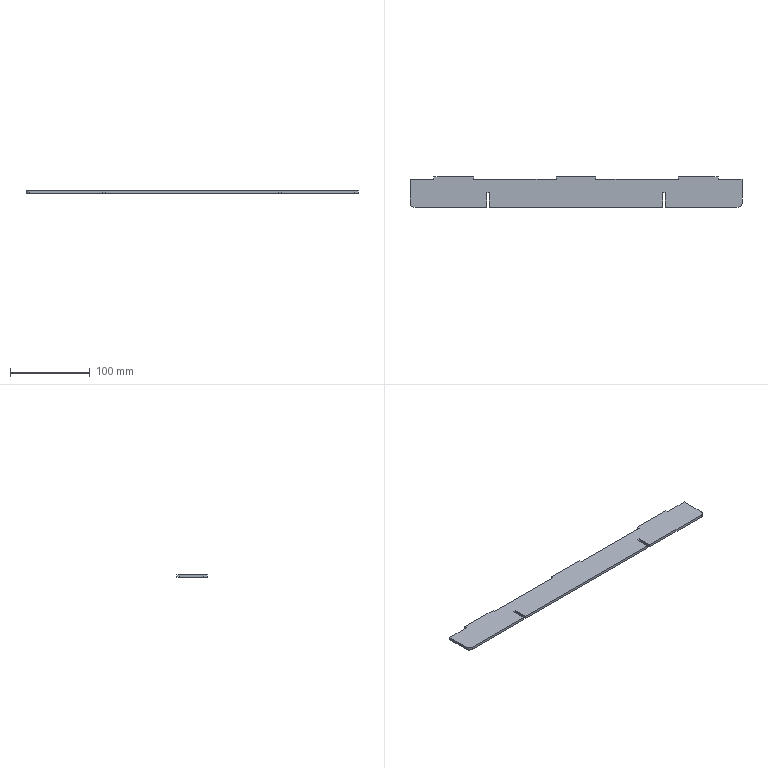Part | SolidWorks | features FlatPattern 1, SMBaseFlange 1, SheetMetal 1 | 1 solid | 28 faces | box 416 x 38 x 3.2 mm | volume 47629 mm3 | plane 26 | cylinder 2 | commonest cylinder face diameters 10 x2
STEP:
#1=CARTESIAN_POINT('',(-198.294,-320.35,0.));
#2=VERTEX_POINT('',#1);
#3=CARTESIAN_POINT('',(-198.294,-350.35,0.));
#4=VERTEX_POINT('',#3);
#5=CARTESIAN_POINT('',(-198.294,-320.35,0.));
#6=DIRECTION('',(0.,-1.,0.));
#7=VECTOR('',#6,1000.);
#8=LINE('',#5,#7);
#9=EDGE_CURVE('',#2,#4,#8,.T.);
#10=ORIENTED_EDGE('',*,*,#9,.F.);
#11=CARTESIAN_POINT('',(-198.294,-320.35,-3.2));
#12=VERTEX_POINT('',#11);
#13=CARTESIAN_POINT('',(-198.294,-320.35,-3.2));
#14=DIRECTION('',(0.,0.,1.));
#15=VECTOR('',#14,1000.);
#16=LINE('',#13,#15);
#17=EDGE_CURVE('',#12,#2,#16,.T.);
#18=ORIENTED_EDGE('',*,*,#17,.F.);
#19=CARTESIAN_POINT('',(-198.294,-350.35,-3.2));
#20=VERTEX_POINT('',#19);
#21=CARTESIAN_POINT('',(-198.294,-320.35,-3.2));
#22=DIRECTION('',(0.,-1.,0.));
#23=VECTOR('',#22,1000.);
#24=LINE('',#21,#23);
#25=EDGE_CURVE('',#12,#20,#24,.T.);
#26=ORIENTED_EDGE('',*,*,#25,.T.);
#27=CARTESIAN_POINT('',(-198.294,-350.35,-3.2));
#28=DIRECTION('',(0.,0.,1.));
#29=VECTOR('',#28,1000.);
#30=LINE('',#27,#29);
#31=EDGE_CURVE('',#20,#4,#30,.T.);
#32=ORIENTED_EDGE('',*,*,#31,.T.);
#33=EDGE_LOOP('',(#10,#18,#26,#32));
#34=FACE_OUTER_BOUND('',#33,.T.);
#35=CARTESIAN_POINT('',(-198.294,-320.35,-3.2));
#36=DIRECTION('',(-1.,0.,0.));
#37=DIRECTION('',(0.,0.,1.));
#38=AXIS2_PLACEMENT_3D('',#35,#36,#37);
#39=PLANE('',#38);
#40=ADVANCED_FACE('',(#34),#39,.T.);
#41=CARTESIAN_POINT('',(-168.294,-320.35,0.));
#42=VERTEX_POINT('',#41);
#43=CARTESIAN_POINT('',(-198.294,-320.35,0.));
#44=DIRECTION('',(-1.,0.,0.));
#45=VECTOR('',#44,1000.);
#46=LINE('',#43,#45);
#47=EDGE_CURVE('',#42,#2,#46,.T.);
#48=ORIENTED_EDGE('',*,*,#47,.F.);
#49=CARTESIAN_POINT('',(-168.294,-320.35,-3.2));
#50=VERTEX_POINT('',#49);
#51=CARTESIAN_POINT('',(-168.294,-320.35,-3.2));
#52=DIRECTION('',(0.,0.,1.));
#53=VECTOR('',#52,1000.);
#54=LINE('',#51,#53);
#55=EDGE_CURVE('',#50,#42,#54,.T.);
#56=ORIENTED_EDGE('',*,*,#55,.F.);
#57=CARTESIAN_POINT('',(-198.294,-320.35,-3.2));
#58=DIRECTION('',(-1.,0.,0.));
#59=VECTOR('',#58,1000.);
#60=LINE('',#57,#59);
#61=EDGE_CURVE('',#50,#12,#60,.T.);
#62=ORIENTED_EDGE('',*,*,#61,.T.);
#63=ORIENTED_EDGE('',*,*,#17,.T.);
#64=EDGE_LOOP('',(#48,#56,#62,#63));
#65=FACE_OUTER_BOUND('',#64,.T.);
#66=CARTESIAN_POINT('',(-198.294,-320.35,-3.2));
#67=DIRECTION('',(0.,1.,0.));
#68=DIRECTION('',(0.,0.,1.));
#69=AXIS2_PLACEMENT_3D('',#66,#67,#68);
#70=PLANE('',#69);
#71=ADVANCED_FACE('',(#65),#70,.T.);
#72=CARTESIAN_POINT('',(-168.294,-317.35,0.));
#73=VERTEX_POINT('',#72);
#74=CARTESIAN_POINT('',(-168.294,-320.35,0.));
#75=DIRECTION('',(0.,-1.,0.));
#76=VECTOR('',#75,1000.);
#77=LINE('',#74,#76);
#78=EDGE_CURVE('',#73,#42,#77,.T.);
#79=ORIENTED_EDGE('',*,*,#78,.F.);
#80=CARTESIAN_POINT('',(-168.294,-317.35,-3.2));
#81=VERTEX_POINT('',#80);
#82=CARTESIAN_POINT('',(-168.294,-317.35,-3.2));
#83=DIRECTION('',(0.,0.,1.));
#84=VECTOR('',#83,1000.);
#85=LINE('',#82,#84);
#86=EDGE_CURVE('',#81,#73,#85,.T.);
#87=ORIENTED_EDGE('',*,*,#86,.F.);
#88=CARTESIAN_POINT('',(-168.294,-320.35,-3.2));
#89=DIRECTION('',(0.,-1.,0.));
#90=VECTOR('',#89,1000.);
#91=LINE('',#88,#90);
#92=EDGE_CURVE('',#81,#50,#91,.T.);
#93=ORIENTED_EDGE('',*,*,#92,.T.);
#94=ORIENTED_EDGE('',*,*,#55,.T.);
#95=EDGE_LOOP('',(#79,#87,#93,#94));
#96=FACE_OUTER_BOUND('',#95,.T.);
#97=CARTESIAN_POINT('',(-168.294,-320.35,-3.2));
#98=DIRECTION('',(-1.,0.,0.));
#99=DIRECTION('',(0.,0.,1.));
#100=AXIS2_PLACEMENT_3D('',#97,#98,#99);
#101=PLANE('',#100);
#102=ADVANCED_FACE('',(#96),#101,.T.);
#103=CARTESIAN_POINT('',(-118.294,-317.35,0.));
#104=VERTEX_POINT('',#103);
#105=CARTESIAN_POINT('',(-168.294,-317.35,0.));
#106=DIRECTION('',(-1.,0.,0.));
#107=VECTOR('',#106,1000.);
#108=LINE('',#105,#107);
#109=EDGE_CURVE('',#104,#73,#108,.T.);
#110=ORIENTED_EDGE('',*,*,#109,.F.);
#111=CARTESIAN_POINT('',(-118.294,-317.35,-3.2));
#112=VERTEX_POINT('',#111);
#113=CARTESIAN_POINT('',(-118.294,-317.35,-3.2));
#114=DIRECTION('',(0.,0.,1.));
#115=VECTOR('',#114,1000.);
#116=LINE('',#113,#115);
#117=EDGE_CURVE('',#112,#104,#116,.T.);
#118=ORIENTED_EDGE('',*,*,#117,.F.);
#119=CARTESIAN_POINT('',(-168.294,-317.35,-3.2));
#120=DIRECTION('',(-1.,0.,0.));
#121=VECTOR('',#120,1000.);
#122=LINE('',#119,#121);
#123=EDGE_CURVE('',#112,#81,#122,.T.);
#124=ORIENTED_EDGE('',*,*,#123,.T.);
#125=ORIENTED_EDGE('',*,*,#86,.T.);
#126=EDGE_LOOP('',(#110,#118,#124,#125));
#127=FACE_OUTER_BOUND('',#126,.T.);
#128=CARTESIAN_POINT('',(-168.294,-317.35,-3.2));
#129=DIRECTION('',(0.,1.,0.));
#130=DIRECTION('',(0.,0.,1.));
#131=AXIS2_PLACEMENT_3D('',#128,#129,#130);
#132=PLANE('',#131);
#133=ADVANCED_FACE('',(#127),#132,.T.);
#134=CARTESIAN_POINT('',(-118.294,-320.35,0.));
#135=VERTEX_POINT('',#134);
#136=CARTESIAN_POINT('',(-118.294,-317.35,0.));
#137=DIRECTION('',(0.,1.,0.));
#138=VECTOR('',#137,1000.);
#139=LINE('',#136,#138);
#140=EDGE_CURVE('',#135,#104,#139,.T.);
#141=ORIENTED_EDGE('',*,*,#140,.F.);
#142=CARTESIAN_POINT('',(-118.294,-320.35,-3.2));
#143=VERTEX_POINT('',#142);
#144=CARTESIAN_POINT('',(-118.294,-320.35,-3.2));
#145=DIRECTION('',(0.,0.,1.));
#146=VECTOR('',#145,1000.);
#147=LINE('',#144,#146);
#148=EDGE_CURVE('',#143,#135,#147,.T.);
#149=ORIENTED_EDGE('',*,*,#148,.F.);
#150=CARTESIAN_POINT('',(-118.294,-317.35,-3.2));
#151=DIRECTION('',(0.,1.,0.));
#152=VECTOR('',#151,1000.);
#153=LINE('',#150,#152);
#154=EDGE_CURVE('',#143,#112,#153,.T.);
#155=ORIENTED_EDGE('',*,*,#154,.T.);
#156=ORIENTED_EDGE('',*,*,#117,.T.);
#157=EDGE_LOOP('',(#141,#149,#155,#156));
#158=FACE_OUTER_BOUND('',#157,.T.);
#159=CARTESIAN_POINT('',(-118.294,-317.35,-3.2));
#160=DIRECTION('',(1.,0.,0.));
#161=DIRECTION('',(0.,1.,0.));
#162=AXIS2_PLACEMENT_3D('',#159,#160,#161);
#163=PLANE('',#162);
#164=ADVANCED_FACE('',(#158),#163,.T.);
#165=CARTESIAN_POINT('',(-15.294,-320.35,0.));
#166=VERTEX_POINT('',#165);
#167=CARTESIAN_POINT('',(-118.294,-320.35,0.));
#168=DIRECTION('',(-1.,0.,0.));
#169=VECTOR('',#168,1000.);
#170=LINE('',#167,#169);
#171=EDGE_CURVE('',#166,#135,#170,.T.);
#172=ORIENTED_EDGE('',*,*,#171,.F.);
#173=CARTESIAN_POINT('',(-15.294,-320.35,-3.2));
#174=VERTEX_POINT('',#173);
#175=CARTESIAN_POINT('',(-15.294,-320.35,-3.2));
#176=DIRECTION('',(0.,0.,1.));
#177=VECTOR('',#176,1000.);
#178=LINE('',#175,#177);
#179=EDGE_CURVE('',#174,#166,#178,.T.);
#180=ORIENTED_EDGE('',*,*,#179,.F.);
#181=CARTESIAN_POINT('',(-118.294,-320.35,-3.2));
#182=DIRECTION('',(-1.,0.,0.));
#183=VECTOR('',#182,1000.);
#184=LINE('',#181,#183);
#185=EDGE_CURVE('',#174,#143,#184,.T.);
#186=ORIENTED_EDGE('',*,*,#185,.T.);
#187=ORIENTED_EDGE('',*,*,#148,.T.);
#188=EDGE_LOOP('',(#172,#180,#186,#187));
#189=FACE_OUTER_BOUND('',#188,.T.);
#190=CARTESIAN_POINT('',(-118.294,-320.35,-3.2));
#191=DIRECTION('',(0.,1.,0.));
#192=DIRECTION('',(0.,0.,1.));
#193=AXIS2_PLACEMENT_3D('',#190,#191,#192);
#194=PLANE('',#193);
#195=ADVANCED_FACE('',(#189),#194,.T.);
#196=CARTESIAN_POINT('',(-15.294,-317.35,0.));
#197=VERTEX_POINT('',#196);
#198=CARTESIAN_POINT('',(-15.294,-320.35,0.));
#199=DIRECTION('',(0.,-1.,0.));
#200=VECTOR('',#199,1000.);
#201=LINE('',#198,#200);
#202=EDGE_CURVE('',#197,#166,#201,.T.);
#203=ORIENTED_EDGE('',*,*,#202,.F.);
#204=CARTESIAN_POINT('',(-15.294,-317.35,-3.2));
#205=VERTEX_POINT('',#204);
#206=CARTESIAN_POINT('',(-15.294,-317.35,-3.2));
#207=DIRECTION('',(0.,0.,1.));
#208=VECTOR('',#207,1000.);
#209=LINE('',#206,#208);
#210=EDGE_CURVE('',#205,#197,#209,.T.);
#211=ORIENTED_EDGE('',*,*,#210,.F.);
#212=CARTESIAN_POINT('',(-15.294,-320.35,-3.2));
#213=DIRECTION('',(0.,-1.,0.));
#214=VECTOR('',#213,1000.);
#215=LINE('',#212,#214);
#216=EDGE_CURVE('',#205,#174,#215,.T.);
#217=ORIENTED_EDGE('',*,*,#216,.T.);
#218=ORIENTED_EDGE('',*,*,#179,.T.);
#219=EDGE_LOOP('',(#203,#211,#217,#218));
#220=FACE_OUTER_BOUND('',#219,.T.);
#221=CARTESIAN_POINT('',(-15.294,-320.35,-3.2));
#222=DIRECTION('',(-1.,0.,0.));
#223=DIRECTION('',(0.,0.,1.));
#224=AXIS2_PLACEMENT_3D('',#221,#222,#223);
#225=PLANE('',#224);
#226=ADVANCED_FACE('',(#220),#225,.T.);
#227=CARTESIAN_POINT('',(34.706,-317.35,0.));
#228=VERTEX_POINT('',#227);
#229=CARTESIAN_POINT('',(-15.294,-317.35,0.));
#230=DIRECTION('',(-1.,0.,0.));
#231=VECTOR('',#230,1000.);
#232=LINE('',#229,#231);
#233=EDGE_CURVE('',#228,#197,#232,.T.);
#234=ORIENTED_EDGE('',*,*,#233,.F.);
#235=CARTESIAN_POINT('',(34.706,-317.35,-3.2));
#236=VERTEX_POINT('',#235);
#237=CARTESIAN_POINT('',(34.706,-317.35,-3.2));
#238=DIRECTION('',(0.,0.,1.));
#239=VECTOR('',#238,1000.);
#240=LINE('',#237,#239);
#241=EDGE_CURVE('',#236,#228,#240,.T.);
#242=ORIENTED_EDGE('',*,*,#241,.F.);
#243=CARTESIAN_POINT('',(-15.294,-317.35,-3.2));
#244=DIRECTION('',(-1.,0.,0.));
#245=VECTOR('',#244,1000.);
#246=LINE('',#243,#245);
#247=EDGE_CURVE('',#236,#205,#246,.T.);
#248=ORIENTED_EDGE('',*,*,#247,.T.);
#249=ORIENTED_EDGE('',*,*,#210,.T.);
#250=EDGE_LOOP('',(#234,#242,#248,#249));
#251=FACE_OUTER_BOUND('',#250,.T.);
#252=CARTESIAN_POINT('',(-15.294,-317.35,-3.2));
#253=DIRECTION('',(0.,1.,0.));
#254=DIRECTION('',(-1.,0.,0.));
#255=AXIS2_PLACEMENT_3D('',#252,#253,#254);
#256=PLANE('',#255);
#257=ADVANCED_FACE('',(#251),#256,.T.);
#258=CARTESIAN_POINT('',(34.706,-320.35,0.));
#259=VERTEX_POINT('',#258);
#260=CARTESIAN_POINT('',(34.706,-317.35,0.));
#261=DIRECTION('',(0.,1.,0.));
#262=VECTOR('',#261,1000.);
#263=LINE('',#260,#262);
#264=EDGE_CURVE('',#259,#228,#263,.T.);
#265=ORIENTED_EDGE('',*,*,#264,.F.);
#266=CARTESIAN_POINT('',(34.706,-320.35,-3.2));
#267=VERTEX_POINT('',#266);
#268=CARTESIAN_POINT('',(34.706,-320.35,-3.2));
#269=DIRECTION('',(0.,0.,1.));
#270=VECTOR('',#269,1000.);
#271=LINE('',#268,#270);
#272=EDGE_CURVE('',#267,#259,#271,.T.);
#273=ORIENTED_EDGE('',*,*,#272,.F.);
#274=CARTESIAN_POINT('',(34.706,-317.35,-3.2));
#275=DIRECTION('',(0.,1.,0.));
#276=VECTOR('',#275,1000.);
#277=LINE('',#274,#276);
#278=EDGE_CURVE('',#267,#236,#277,.T.);
#279=ORIENTED_EDGE('',*,*,#278,.T.);
#280=ORIENTED_EDGE('',*,*,#241,.T.);
#281=EDGE_LOOP('',(#265,#273,#279,#280));
#282=FACE_OUTER_BOUND('',#281,.T.);
#283=CARTESIAN_POINT('',(34.706,-317.35,-3.2));
#284=DIRECTION('',(1.,0.,0.));
#285=DIRECTION('',(0.,0.,-1.));
#286=AXIS2_PLACEMENT_3D('',#283,#284,#285);
#287=PLANE('',#286);
#288=ADVANCED_FACE('',(#282),#287,.T.);
#289=CARTESIAN_POINT('',(137.706,-320.35,0.));
#290=VERTEX_POINT('',#289);
#291=CARTESIAN_POINT('',(34.706,-320.35,0.));
#292=DIRECTION('',(-1.,0.,0.));
#293=VECTOR('',#292,1000.);
#294=LINE('',#291,#293);
#295=EDGE_CURVE('',#290,#259,#294,.T.);
#296=ORIENTED_EDGE('',*,*,#295,.F.);
#297=CARTESIAN_POINT('',(137.706,-320.35,-3.2));
#298=VERTEX_POINT('',#297);
#299=CARTESIAN_POINT('',(137.706,-320.35,-3.2));
#300=DIRECTION('',(0.,0.,1.));
#301=VECTOR('',#300,1000.);
#302=LINE('',#299,#301);
#303=EDGE_CURVE('',#298,#290,#302,.T.);
#304=ORIENTED_EDGE('',*,*,#303,.F.);
#305=CARTESIAN_POINT('',(34.706,-320.35,-3.2));
#306=DIRECTION('',(-1.,0.,0.));
#307=VECTOR('',#306,1000.);
#308=LINE('',#305,#307);
#309=EDGE_CURVE('',#298,#267,#308,.T.);
#310=ORIENTED_EDGE('',*,*,#309,.T.);
#311=ORIENTED_EDGE('',*,*,#272,.T.);
#312=EDGE_LOOP('',(#296,#304,#310,#311));
#313=FACE_OUTER_BOUND('',#312,.T.);
#314=CARTESIAN_POINT('',(34.706,-320.35,-3.2));
#315=DIRECTION('',(0.,1.,0.));
#316=DIRECTION('',(-1.,0.,0.));
#317=AXIS2_PLACEMENT_3D('',#314,#315,#316);
#318=PLANE('',#317);
#319=ADVANCED_FACE('',(#313),#318,.T.);
#320=CARTESIAN_POINT('',(137.706,-317.35,0.));
#321=VERTEX_POINT('',#320);
#322=CARTESIAN_POINT('',(137.706,-317.35,0.));
#323=DIRECTION('',(0.,-1.,0.));
#324=VECTOR('',#323,1000.);
#325=LINE('',#322,#324);
#326=EDGE_CURVE('',#321,#290,#325,.T.);
#327=ORIENTED_EDGE('',*,*,#326,.F.);
#328=CARTESIAN_POINT('',(137.706,-317.35,-3.2));
#329=VERTEX_POINT('',#328);
#330=CARTESIAN_POINT('',(137.706,-317.35,-3.2));
#331=DIRECTION('',(0.,0.,1.));
#332=VECTOR('',#331,1000.);
#333=LINE('',#330,#332);
#334=EDGE_CURVE('',#329,#321,#333,.T.);
#335=ORIENTED_EDGE('',*,*,#334,.F.);
#336=CARTESIAN_POINT('',(137.706,-317.35,-3.2));
#337=DIRECTION('',(0.,-1.,0.));
#338=VECTOR('',#337,1000.);
#339=LINE('',#336,#338);
#340=EDGE_CURVE('',#329,#298,#339,.T.);
#341=ORIENTED_EDGE('',*,*,#340,.T.);
#342=ORIENTED_EDGE('',*,*,#303,.T.);
#343=EDGE_LOOP('',(#327,#335,#341,#342));
#344=FACE_OUTER_BOUND('',#343,.T.);
#345=CARTESIAN_POINT('',(137.706,-317.35,-3.2));
#346=DIRECTION('',(-1.,0.,0.));
#347=DIRECTION('',(0.,0.,1.));
#348=AXIS2_PLACEMENT_3D('',#345,#346,#347);
#349=PLANE('',#348);
#350=ADVANCED_FACE('',(#344),#349,.T.);
#351=CARTESIAN_POINT('',(187.706,-317.35,0.));
#352=VERTEX_POINT('',#351);
#353=CARTESIAN_POINT('',(187.706,-317.35,0.));
#354=DIRECTION('',(-1.,0.,0.));
#355=VECTOR('',#354,1000.);
#356=LINE('',#353,#355);
#357=EDGE_CURVE('',#352,#321,#356,.T.);
#358=ORIENTED_EDGE('',*,*,#357,.F.);
#359=CARTESIAN_POINT('',(187.706,-317.35,-3.2));
#360=VERTEX_POINT('',#359);
#361=CARTESIAN_POINT('',(187.706,-317.35,-3.2));
#362=DIRECTION('',(0.,0.,1.));
#363=VECTOR('',#362,1000.);
#364=LINE('',#361,#363);
#365=EDGE_CURVE('',#360,#352,#364,.T.);
#366=ORIENTED_EDGE('',*,*,#365,.F.);
#367=CARTESIAN_POINT('',(187.706,-317.35,-3.2));
#368=DIRECTION('',(-1.,0.,0.));
#369=VECTOR('',#368,1000.);
#370=LINE('',#367,#369);
#371=EDGE_CURVE('',#360,#329,#370,.T.);
#372=ORIENTED_EDGE('',*,*,#371,.T.);
#373=ORIENTED_EDGE('',*,*,#334,.T.);
#374=EDGE_LOOP('',(#358,#366,#372,#373));
#375=FACE_OUTER_BOUND('',#374,.T.);
#376=CARTESIAN_POINT('',(187.706,-317.35,-3.2));
#377=DIRECTION('',(0.,1.,0.));
#378=DIRECTION('',(0.,0.,1.));
#379=AXIS2_PLACEMENT_3D('',#376,#377,#378);
#380=PLANE('',#379);
#381=ADVANCED_FACE('',(#375),#380,.T.);
#382=CARTESIAN_POINT('',(187.706,-320.35,0.));
#383=VERTEX_POINT('',#382);
#384=CARTESIAN_POINT('',(187.706,-320.35,0.));
#385=DIRECTION('',(0.,1.,0.));
#386=VECTOR('',#385,1000.);
#387=LINE('',#384,#386);
#388=EDGE_CURVE('',#383,#352,#387,.T.);
#389=ORIENTED_EDGE('',*,*,#388,.F.);
#390=CARTESIAN_POINT('',(187.706,-320.35,-3.2));
#391=VERTEX_POINT('',#390);
#392=CARTESIAN_POINT('',(187.706,-320.35,-3.2));
#393=DIRECTION('',(0.,0.,1.));
#394=VECTOR('',#393,1000.);
#395=LINE('',#392,#394);
#396=EDGE_CURVE('',#391,#383,#395,.T.);
#397=ORIENTED_EDGE('',*,*,#396,.F.);
#398=CARTESIAN_POINT('',(187.706,-320.35,-3.2));
#399=DIRECTION('',(0.,1.,0.));
#400=VECTOR('',#399,1000.);
#401=LINE('',#398,#400);
#402=EDGE_CURVE('',#391,#360,#401,.T.);
#403=ORIENTED_EDGE('',*,*,#402,.T.);
#404=ORIENTED_EDGE('',*,*,#365,.T.);
#405=EDGE_LOOP('',(#389,#397,#403,#404));
#406=FACE_OUTER_BOUND('',#405,.T.);
#407=CARTESIAN_POINT('',(187.706,-320.35,-3.2));
#408=DIRECTION('',(1.,0.,0.));
#409=DIRECTION('',(0.,0.,-1.));
#410=AXIS2_PLACEMENT_3D('',#407,#408,#409);
#411=PLANE('',#410);
#412=ADVANCED_FACE('',(#406),#411,.T.);
#413=CARTESIAN_POINT('',(217.706,-320.35,0.));
#414=VERTEX_POINT('',#413);
#415=CARTESIAN_POINT('',(187.706,-320.35,0.));
#416=DIRECTION('',(-1.,0.,0.));
#417=VECTOR('',#416,1000.);
#418=LINE('',#415,#417);
#419=EDGE_CURVE('',#414,#383,#418,.T.);
#420=ORIENTED_EDGE('',*,*,#419,.F.);
#421=CARTESIAN_POINT('',(217.706,-320.35,-3.2));
#422=VERTEX_POINT('',#421);
#423=CARTESIAN_POINT('',(217.706,-320.35,-3.2));
#424=DIRECTION('',(0.,0.,1.));
#425=VECTOR('',#424,1000.);
#426=LINE('',#423,#425);
#427=EDGE_CURVE('',#422,#414,#426,.T.);
#428=ORIENTED_EDGE('',*,*,#427,.F.);
#429=CARTESIAN_POINT('',(187.706,-320.35,-3.2));
#430=DIRECTION('',(-1.,0.,0.));
#431=VECTOR('',#430,1000.);
#432=LINE('',#429,#431);
#433=EDGE_CURVE('',#422,#391,#432,.T.);
#434=ORIENTED_EDGE('',*,*,#433,.T.);
#435=ORIENTED_EDGE('',*,*,#396,.T.);
#436=EDGE_LOOP('',(#420,#428,#434,#435));
#437=FACE_OUTER_BOUND('',#436,.T.);
#438=CARTESIAN_POINT('',(187.706,-320.35,-3.2));
#439=DIRECTION('',(0.,1.,0.));
#440=DIRECTION('',(0.,0.,1.));
#441=AXIS2_PLACEMENT_3D('',#438,#439,#440);
#442=PLANE('',#441);
#443=ADVANCED_FACE('',(#437),#442,.T.);
#444=CARTESIAN_POINT('',(217.706,-350.35,0.));
#445=VERTEX_POINT('',#444);
#446=CARTESIAN_POINT('',(217.706,-320.35,0.));
#447=DIRECTION('',(0.,1.,0.));
#448=VECTOR('',#447,1000.);
#449=LINE('',#446,#448);
#450=EDGE_CURVE('',#445,#414,#449,.T.);
#451=ORIENTED_EDGE('',*,*,#450,.F.);
#452=CARTESIAN_POINT('',(217.706,-350.35,-3.2));
#453=VERTEX_POINT('',#452);
#454=CARTESIAN_POINT('',(217.706,-350.35,-3.2));
#455=DIRECTION('',(0.,0.,1.));
#456=VECTOR('',#455,1000.);
#457=LINE('',#454,#456);
#458=EDGE_CURVE('',#453,#445,#457,.T.);
#459=ORIENTED_EDGE('',*,*,#458,.F.);
#460=CARTESIAN_POINT('',(217.706,-320.35,-3.2));
#461=DIRECTION('',(0.,1.,0.));
#462=VECTOR('',#461,1000.);
#463=LINE('',#460,#462);
#464=EDGE_CURVE('',#453,#422,#463,.T.);
#465=ORIENTED_EDGE('',*,*,#464,.T.);
#466=ORIENTED_EDGE('',*,*,#427,.T.);
#467=EDGE_LOOP('',(#451,#459,#465,#466));
#468=FACE_OUTER_BOUND('',#467,.T.);
#469=CARTESIAN_POINT('',(217.706,-320.35,-3.2));
#470=DIRECTION('',(1.,0.,0.));
#471=DIRECTION('',(0.,1.,0.));
#472=AXIS2_PLACEMENT_3D('',#469,#470,#471);
#473=PLANE('',#472);
#474=ADVANCED_FACE('',(#468),#473,.T.);
#475=CARTESIAN_POINT('',(212.706,-355.35,0.));
#476=VERTEX_POINT('',#475);
#477=CARTESIAN_POINT('',(212.706,-350.35,0.));
#478=DIRECTION('',(0.,0.,1.));
#479=DIRECTION('',(1.,0.,0.));
#480=AXIS2_PLACEMENT_3D('',#477,#478,#479);
#481=CIRCLE('',#480,5.);
#482=EDGE_CURVE('',#476,#445,#481,.T.);
#483=ORIENTED_EDGE('',*,*,#482,.F.);
#484=CARTESIAN_POINT('',(212.706,-355.35,-3.2));
#485=VERTEX_POINT('',#484);
#486=CARTESIAN_POINT('',(212.706,-355.35,-3.2));
#487=DIRECTION('',(0.,0.,1.));
#488=VECTOR('',#487,1000.);
#489=LINE('',#486,#488);
#490=EDGE_CURVE('',#485,#476,#489,.T.);
#491=ORIENTED_EDGE('',*,*,#490,.F.);
#492=CARTESIAN_POINT('',(212.706,-350.35,-3.2));
#493=DIRECTION('',(0.,0.,1.));
#494=DIRECTION('',(1.,0.,0.));
#495=AXIS2_PLACEMENT_3D('',#492,#493,#494);
#496=CIRCLE('',#495,5.);
#497=EDGE_CURVE('',#485,#453,#496,.T.);
#498=ORIENTED_EDGE('',*,*,#497,.T.);
#499=ORIENTED_EDGE('',*,*,#458,.T.);
#500=EDGE_LOOP('',(#483,#491,#498,#499));
#501=FACE_OUTER_BOUND('',#500,.T.);
#502=CARTESIAN_POINT('',(212.706,-350.35,-3.2));
#503=DIRECTION('',(0.,0.,1.));
#504=DIRECTION('',(1.,0.,0.));
#505=AXIS2_PLACEMENT_3D('',#502,#503,#504);
#506=CYLINDRICAL_SURFACE('',#505,5.);
#507=ADVANCED_FACE('',(#501),#506,.T.);
#508=CARTESIAN_POINT('',(121.306,-355.35,0.));
#509=VERTEX_POINT('',#508);
#510=CARTESIAN_POINT('',(121.306,-355.35,0.));
#511=DIRECTION('',(1.,0.,0.));
#512=VECTOR('',#511,1000.);
#513=LINE('',#510,#512);
#514=EDGE_CURVE('',#509,#476,#513,.T.);
#515=ORIENTED_EDGE('',*,*,#514,.F.);
#516=CARTESIAN_POINT('',(121.306,-355.35,-3.2));
#517=VERTEX_POINT('',#516);
#518=CARTESIAN_POINT('',(121.306,-355.35,-3.2));
#519=DIRECTION('',(0.,0.,1.));
#520=VECTOR('',#519,1000.);
#521=LINE('',#518,#520);
#522=EDGE_CURVE('',#517,#509,#521,.T.);
#523=ORIENTED_EDGE('',*,*,#522,.F.);
#524=CARTESIAN_POINT('',(121.306,-355.35,-3.2));
#525=DIRECTION('',(1.,0.,0.));
#526=VECTOR('',#525,1000.);
#527=LINE('',#524,#526);
#528=EDGE_CURVE('',#517,#485,#527,.T.);
#529=ORIENTED_EDGE('',*,*,#528,.T.);
#530=ORIENTED_EDGE('',*,*,#490,.T.);
#531=EDGE_LOOP('',(#515,#523,#529,#530));
#532=FACE_OUTER_BOUND('',#531,.T.);
#533=CARTESIAN_POINT('',(121.306,-355.35,-3.2));
#534=DIRECTION('',(0.,-1.,0.));
#535=DIRECTION('',(1.,0.,0.));
#536=AXIS2_PLACEMENT_3D('',#533,#534,#535);
#537=PLANE('',#536);
#538=ADVANCED_FACE('',(#532),#537,.T.);
#539=CARTESIAN_POINT('',(121.306,-337.35,0.));
#540=VERTEX_POINT('',#539);
#541=CARTESIAN_POINT('',(121.306,-337.35,0.));
#542=DIRECTION('',(0.,-1.,0.));
#543=VECTOR('',#542,1000.);
#544=LINE('',#541,#543);
#545=EDGE_CURVE('',#540,#509,#544,.T.);
#546=ORIENTED_EDGE('',*,*,#545,.F.);
#547=CARTESIAN_POINT('',(121.306,-337.35,-3.2));
#548=VERTEX_POINT('',#547);
#549=CARTESIAN_POINT('',(121.306,-337.35,-3.2));
#550=DIRECTION('',(0.,0.,1.));
#551=VECTOR('',#550,1000.);
#552=LINE('',#549,#551);
#553=EDGE_CURVE('',#548,#540,#552,.T.);
#554=ORIENTED_EDGE('',*,*,#553,.F.);
#555=CARTESIAN_POINT('',(121.306,-337.35,-3.2));
#556=DIRECTION('',(0.,-1.,0.));
#557=VECTOR('',#556,1000.);
#558=LINE('',#555,#557);
#559=EDGE_CURVE('',#548,#517,#558,.T.);
#560=ORIENTED_EDGE('',*,*,#559,.T.);
#561=ORIENTED_EDGE('',*,*,#522,.T.);
#562=EDGE_LOOP('',(#546,#554,#560,#561));
#563=FACE_OUTER_BOUND('',#562,.T.);
#564=CARTESIAN_POINT('',(121.306,-337.35,-3.2));
#565=DIRECTION('',(-1.,0.,0.));
#566=DIRECTION('',(0.,0.,1.));
#567=AXIS2_PLACEMENT_3D('',#564,#565,#566);
#568=PLANE('',#567);
#569=ADVANCED_FACE('',(#563),#568,.T.);
#570=CARTESIAN_POINT('',(118.106,-337.35,0.));
#571=VERTEX_POINT('',#570);
#572=CARTESIAN_POINT('',(118.106,-337.35,0.));
#573=DIRECTION('',(1.,0.,0.));
#574=VECTOR('',#573,1000.);
#575=LINE('',#572,#574);
#576=EDGE_CURVE('',#571,#540,#575,.T.);
#577=ORIENTED_EDGE('',*,*,#576,.F.);
#578=CARTESIAN_POINT('',(118.106,-337.35,-3.2));
#579=VERTEX_POINT('',#578);
#580=CARTESIAN_POINT('',(118.106,-337.35,-3.2));
#581=DIRECTION('',(0.,0.,1.));
#582=VECTOR('',#581,1000.);
#583=LINE('',#580,#582);
#584=EDGE_CURVE('',#579,#571,#583,.T.);
#585=ORIENTED_EDGE('',*,*,#584,.F.);
#586=CARTESIAN_POINT('',(118.106,-337.35,-3.2));
#587=DIRECTION('',(1.,0.,0.));
#588=VECTOR('',#587,1000.);
#589=LINE('',#586,#588);
#590=EDGE_CURVE('',#579,#548,#589,.T.);
#591=ORIENTED_EDGE('',*,*,#590,.T.);
#592=ORIENTED_EDGE('',*,*,#553,.T.);
#593=EDGE_LOOP('',(#577,#585,#591,#592));
#594=FACE_OUTER_BOUND('',#593,.T.);
#595=CARTESIAN_POINT('',(118.106,-337.35,-3.2));
#596=DIRECTION('',(0.,-1.,0.));
#597=DIRECTION('',(0.,0.,-1.));
#598=AXIS2_PLACEMENT_3D('',#595,#596,#597);
#599=PLANE('',#598);
#600=ADVANCED_FACE('',(#594),#599,.T.);
#601=CARTESIAN_POINT('',(118.106,-355.35,0.));
#602=VERTEX_POINT('',#601);
#603=CARTESIAN_POINT('',(118.106,-355.35,0.));
#604=DIRECTION('',(0.,1.,0.));
#605=VECTOR('',#604,1000.);
#606=LINE('',#603,#605);
#607=EDGE_CURVE('',#602,#571,#606,.T.);
#608=ORIENTED_EDGE('',*,*,#607,.F.);
#609=CARTESIAN_POINT('',(118.106,-355.35,-3.2));
#610=VERTEX_POINT('',#609);
#611=CARTESIAN_POINT('',(118.106,-355.35,-3.2));
#612=DIRECTION('',(0.,0.,1.));
#613=VECTOR('',#612,1000.);
#614=LINE('',#611,#613);
#615=EDGE_CURVE('',#610,#602,#614,.T.);
#616=ORIENTED_EDGE('',*,*,#615,.F.);
#617=CARTESIAN_POINT('',(118.106,-355.35,-3.2));
#618=DIRECTION('',(0.,1.,0.));
#619=VECTOR('',#618,1000.);
#620=LINE('',#617,#619);
#621=EDGE_CURVE('',#610,#579,#620,.T.);
#622=ORIENTED_EDGE('',*,*,#621,.T.);
#623=ORIENTED_EDGE('',*,*,#584,.T.);
#624=EDGE_LOOP('',(#608,#616,#622,#623));
#625=FACE_OUTER_BOUND('',#624,.T.);
#626=CARTESIAN_POINT('',(118.106,-355.35,-3.2));
#627=DIRECTION('',(1.,0.,0.));
#628=DIRECTION('',(0.,0.,-1.));
#629=AXIS2_PLACEMENT_3D('',#626,#627,#628);
#630=PLANE('',#629);
#631=ADVANCED_FACE('',(#625),#630,.T.);
#632=CARTESIAN_POINT('',(-98.694,-355.35,0.));
#633=VERTEX_POINT('',#632);
#634=CARTESIAN_POINT('',(-98.694,-355.35,0.));
#635=DIRECTION('',(1.,0.,0.));
#636=VECTOR('',#635,1000.);
#637=LINE('',#634,#636);
#638=EDGE_CURVE('',#633,#602,#637,.T.);
#639=ORIENTED_EDGE('',*,*,#638,.F.);
#640=CARTESIAN_POINT('',(-98.694,-355.35,-3.2));
#641=VERTEX_POINT('',#640);
#642=CARTESIAN_POINT('',(-98.694,-355.35,-3.2));
#643=DIRECTION('',(0.,0.,1.));
#644=VECTOR('',#643,1000.);
#645=LINE('',#642,#644);
#646=EDGE_CURVE('',#641,#633,#645,.T.);
#647=ORIENTED_EDGE('',*,*,#646,.F.);
#648=CARTESIAN_POINT('',(-98.694,-355.35,-3.2));
#649=DIRECTION('',(1.,0.,0.));
#650=VECTOR('',#649,1000.);
#651=LINE('',#648,#650);
#652=EDGE_CURVE('',#641,#610,#651,.T.);
#653=ORIENTED_EDGE('',*,*,#652,.T.);
#654=ORIENTED_EDGE('',*,*,#615,.T.);
#655=EDGE_LOOP('',(#639,#647,#653,#654));
#656=FACE_OUTER_BOUND('',#655,.T.);
#657=CARTESIAN_POINT('',(-98.694,-355.35,-3.2));
#658=DIRECTION('',(0.,-1.,0.));
#659=DIRECTION('',(0.,0.,-1.));
#660=AXIS2_PLACEMENT_3D('',#657,#658,#659);
#661=PLANE('',#660);
#662=ADVANCED_FACE('',(#656),#661,.T.);
#663=CARTESIAN_POINT('',(-98.694,-337.35,0.));
#664=VERTEX_POINT('',#663);
#665=CARTESIAN_POINT('',(-98.694,-337.35,0.));
#666=DIRECTION('',(0.,-1.,0.));
#667=VECTOR('',#666,1000.);
#668=LINE('',#665,#667);
#669=EDGE_CURVE('',#664,#633,#668,.T.);
#670=ORIENTED_EDGE('',*,*,#669,.F.);
#671=CARTESIAN_POINT('',(-98.694,-337.35,-3.2));
#672=VERTEX_POINT('',#671);
#673=CARTESIAN_POINT('',(-98.694,-337.35,-3.2));
#674=DIRECTION('',(0.,0.,1.));
#675=VECTOR('',#674,1000.);
#676=LINE('',#673,#675);
#677=EDGE_CURVE('',#672,#664,#676,.T.);
#678=ORIENTED_EDGE('',*,*,#677,.F.);
#679=CARTESIAN_POINT('',(-98.694,-337.35,-3.2));
#680=DIRECTION('',(0.,-1.,0.));
#681=VECTOR('',#680,1000.);
#682=LINE('',#679,#681);
#683=EDGE_CURVE('',#672,#641,#682,.T.);
#684=ORIENTED_EDGE('',*,*,#683,.T.);
#685=ORIENTED_EDGE('',*,*,#646,.T.);
#686=EDGE_LOOP('',(#670,#678,#684,#685));
#687=FACE_OUTER_BOUND('',#686,.T.);
#688=CARTESIAN_POINT('',(-98.694,-337.35,-3.2));
#689=DIRECTION('',(-1.,0.,0.));
#690=DIRECTION('',(0.,0.,1.));
#691=AXIS2_PLACEMENT_3D('',#688,#689,#690);
#692=PLANE('',#691);
#693=ADVANCED_FACE('',(#687),#692,.T.);
#694=CARTESIAN_POINT('',(-101.894,-337.35,0.));
#695=VERTEX_POINT('',#694);
#696=CARTESIAN_POINT('',(-101.894,-337.35,0.));
#697=DIRECTION('',(1.,0.,0.));
#698=VECTOR('',#697,1000.);
#699=LINE('',#696,#698);
#700=EDGE_CURVE('',#695,#664,#699,.T.);
#701=ORIENTED_EDGE('',*,*,#700,.F.);
#702=CARTESIAN_POINT('',(-101.894,-337.35,-3.2));
#703=VERTEX_POINT('',#702);
#704=CARTESIAN_POINT('',(-101.894,-337.35,-3.2));
#705=DIRECTION('',(0.,0.,1.));
#706=VECTOR('',#705,1000.);
#707=LINE('',#704,#706);
#708=EDGE_CURVE('',#703,#695,#707,.T.);
#709=ORIENTED_EDGE('',*,*,#708,.F.);
#710=CARTESIAN_POINT('',(-101.894,-337.35,-3.2));
#711=DIRECTION('',(1.,0.,0.));
#712=VECTOR('',#711,1000.);
#713=LINE('',#710,#712);
#714=EDGE_CURVE('',#703,#672,#713,.T.);
#715=ORIENTED_EDGE('',*,*,#714,.T.);
#716=ORIENTED_EDGE('',*,*,#677,.T.);
#717=EDGE_LOOP('',(#701,#709,#715,#716));
#718=FACE_OUTER_BOUND('',#717,.T.);
#719=CARTESIAN_POINT('',(-101.894,-337.35,-3.2));
#720=DIRECTION('',(0.,-1.,0.));
#721=DIRECTION('',(0.,0.,-1.));
#722=AXIS2_PLACEMENT_3D('',#719,#720,#721);
#723=PLANE('',#722);
#724=ADVANCED_FACE('',(#718),#723,.T.);
#725=CARTESIAN_POINT('',(-101.894,-355.35,0.));
#726=VERTEX_POINT('',#725);
#727=CARTESIAN_POINT('',(-101.894,-355.35,0.));
#728=DIRECTION('',(0.,1.,0.));
#729=VECTOR('',#728,1000.);
#730=LINE('',#727,#729);
#731=EDGE_CURVE('',#726,#695,#730,.T.);
#732=ORIENTED_EDGE('',*,*,#731,.F.);
#733=CARTESIAN_POINT('',(-101.894,-355.35,-3.2));
#734=VERTEX_POINT('',#733);
#735=CARTESIAN_POINT('',(-101.894,-355.35,-3.2));
#736=DIRECTION('',(0.,0.,1.));
#737=VECTOR('',#736,1000.);
#738=LINE('',#735,#737);
#739=EDGE_CURVE('',#734,#726,#738,.T.);
#740=ORIENTED_EDGE('',*,*,#739,.F.);
#741=CARTESIAN_POINT('',(-101.894,-355.35,-3.2));
#742=DIRECTION('',(0.,1.,0.));
#743=VECTOR('',#742,1000.);
#744=LINE('',#741,#743);
#745=EDGE_CURVE('',#734,#703,#744,.T.);
#746=ORIENTED_EDGE('',*,*,#745,.T.);
#747=ORIENTED_EDGE('',*,*,#708,.T.);
#748=EDGE_LOOP('',(#732,#740,#746,#747));
#749=FACE_OUTER_BOUND('',#748,.T.);
#750=CARTESIAN_POINT('',(-101.894,-355.35,-3.2));
#751=DIRECTION('',(1.,0.,0.));
#752=DIRECTION('',(0.,0.,-1.));
#753=AXIS2_PLACEMENT_3D('',#750,#751,#752);
#754=PLANE('',#753);
#755=ADVANCED_FACE('',(#749),#754,.T.);
#756=CARTESIAN_POINT('',(-193.294,-355.35,0.));
#757=VERTEX_POINT('',#756);
#758=CARTESIAN_POINT('',(-193.294,-355.35,0.));
#759=DIRECTION('',(1.,0.,0.));
#760=VECTOR('',#759,1000.);
#761=LINE('',#758,#760);
#762=EDGE_CURVE('',#757,#726,#761,.T.);
#763=ORIENTED_EDGE('',*,*,#762,.F.);
#764=CARTESIAN_POINT('',(-193.294,-355.35,-3.2));
#765=VERTEX_POINT('',#764);
#766=CARTESIAN_POINT('',(-193.294,-355.35,-3.2));
#767=DIRECTION('',(0.,0.,1.));
#768=VECTOR('',#767,1000.);
#769=LINE('',#766,#768);
#770=EDGE_CURVE('',#765,#757,#769,.T.);
#771=ORIENTED_EDGE('',*,*,#770,.F.);
#772=CARTESIAN_POINT('',(-193.294,-355.35,-3.2));
#773=DIRECTION('',(1.,0.,0.));
#774=VECTOR('',#773,1000.);
#775=LINE('',#772,#774);
#776=EDGE_CURVE('',#765,#734,#775,.T.);
#777=ORIENTED_EDGE('',*,*,#776,.T.);
#778=ORIENTED_EDGE('',*,*,#739,.T.);
#779=EDGE_LOOP('',(#763,#771,#777,#778));
#780=FACE_OUTER_BOUND('',#779,.T.);
#781=CARTESIAN_POINT('',(-193.294,-355.35,-3.2));
#782=DIRECTION('',(0.,-1.,0.));
#783=DIRECTION('',(1.,0.,0.));
#784=AXIS2_PLACEMENT_3D('',#781,#782,#783);
#785=PLANE('',#784);
#786=ADVANCED_FACE('',(#780),#785,.T.);
#787=CARTESIAN_POINT('',(-193.294,-350.35,0.));
#788=DIRECTION('',(0.,0.,1.));
#789=DIRECTION('',(1.,0.,0.));
#790=AXIS2_PLACEMENT_3D('',#787,#788,#789);
#791=CIRCLE('',#790,5.);
#792=EDGE_CURVE('',#4,#757,#791,.T.);
#793=ORIENTED_EDGE('',*,*,#792,.F.);
#794=ORIENTED_EDGE('',*,*,#31,.F.);
#795=CARTESIAN_POINT('',(-193.294,-350.35,-3.2));
#796=DIRECTION('',(0.,0.,1.));
#797=DIRECTION('',(1.,0.,0.));
#798=AXIS2_PLACEMENT_3D('',#795,#796,#797);
#799=CIRCLE('',#798,5.);
#800=EDGE_CURVE('',#20,#765,#799,.T.);
#801=ORIENTED_EDGE('',*,*,#800,.T.);
#802=ORIENTED_EDGE('',*,*,#770,.T.);
#803=EDGE_LOOP('',(#793,#794,#801,#802));
#804=FACE_OUTER_BOUND('',#803,.T.);
#805=CARTESIAN_POINT('',(-193.294,-350.35,-3.2));
#806=DIRECTION('',(0.,0.,1.));
#807=DIRECTION('',(1.,0.,0.));
#808=AXIS2_PLACEMENT_3D('',#805,#806,#807);
#809=CYLINDRICAL_SURFACE('',#808,5.);
#810=ADVANCED_FACE('',(#804),#809,.T.);
#811=ORIENTED_EDGE('',*,*,#25,.F.);
#812=ORIENTED_EDGE('',*,*,#61,.F.);
#813=ORIENTED_EDGE('',*,*,#92,.F.);
#814=ORIENTED_EDGE('',*,*,#123,.F.);
#815=ORIENTED_EDGE('',*,*,#154,.F.);
#816=ORIENTED_EDGE('',*,*,#185,.F.);
#817=ORIENTED_EDGE('',*,*,#216,.F.);
#818=ORIENTED_EDGE('',*,*,#247,.F.);
#819=ORIENTED_EDGE('',*,*,#278,.F.);
#820=ORIENTED_EDGE('',*,*,#309,.F.);
#821=ORIENTED_EDGE('',*,*,#340,.F.);
#822=ORIENTED_EDGE('',*,*,#371,.F.);
#823=ORIENTED_EDGE('',*,*,#402,.F.);
#824=ORIENTED_EDGE('',*,*,#433,.F.);
#825=ORIENTED_EDGE('',*,*,#464,.F.);
#826=ORIENTED_EDGE('',*,*,#497,.F.);
#827=ORIENTED_EDGE('',*,*,#528,.F.);
#828=ORIENTED_EDGE('',*,*,#559,.F.);
#829=ORIENTED_EDGE('',*,*,#590,.F.);
#830=ORIENTED_EDGE('',*,*,#621,.F.);
#831=ORIENTED_EDGE('',*,*,#652,.F.);
#832=ORIENTED_EDGE('',*,*,#683,.F.);
#833=ORIENTED_EDGE('',*,*,#714,.F.);
#834=ORIENTED_EDGE('',*,*,#745,.F.);
#835=ORIENTED_EDGE('',*,*,#776,.F.);
#836=ORIENTED_EDGE('',*,*,#800,.F.);
#837=EDGE_LOOP('',(#811,#812,#813,#814,#815,#816,#817,#818,#819,#820,#821,#822,#823,#824,#825,#826,#827,#828,#829,#830,#831,#832,#833,#834,#835,#836));
#838=FACE_OUTER_BOUND('',#837,.T.);
#839=CARTESIAN_POINT('',(-193.294,-350.35,-3.2));
#840=DIRECTION('',(0.,0.,1.));
#841=DIRECTION('',(1.,0.,0.));
#842=AXIS2_PLACEMENT_3D('',#839,#840,#841);
#843=PLANE('',#842);
#844=ADVANCED_FACE('',(#838),#843,.F.);
#845=ORIENTED_EDGE('',*,*,#9,.T.);
#846=ORIENTED_EDGE('',*,*,#792,.T.);
#847=ORIENTED_EDGE('',*,*,#762,.T.);
#848=ORIENTED_EDGE('',*,*,#731,.T.);
#849=ORIENTED_EDGE('',*,*,#700,.T.);
#850=ORIENTED_EDGE('',*,*,#669,.T.);
#851=ORIENTED_EDGE('',*,*,#638,.T.);
#852=ORIENTED_EDGE('',*,*,#607,.T.);
#853=ORIENTED_EDGE('',*,*,#576,.T.);
#854=ORIENTED_EDGE('',*,*,#545,.T.);
#855=ORIENTED_EDGE('',*,*,#514,.T.);
#856=ORIENTED_EDGE('',*,*,#482,.T.);
#857=ORIENTED_EDGE('',*,*,#450,.T.);
#858=ORIENTED_EDGE('',*,*,#419,.T.);
#859=ORIENTED_EDGE('',*,*,#388,.T.);
#860=ORIENTED_EDGE('',*,*,#357,.T.);
#861=ORIENTED_EDGE('',*,*,#326,.T.);
#862=ORIENTED_EDGE('',*,*,#295,.T.);
#863=ORIENTED_EDGE('',*,*,#264,.T.);
#864=ORIENTED_EDGE('',*,*,#233,.T.);
#865=ORIENTED_EDGE('',*,*,#202,.T.);
#866=ORIENTED_EDGE('',*,*,#171,.T.);
#867=ORIENTED_EDGE('',*,*,#140,.T.);
#868=ORIENTED_EDGE('',*,*,#109,.T.);
#869=ORIENTED_EDGE('',*,*,#78,.T.);
#870=ORIENTED_EDGE('',*,*,#47,.T.);
#871=EDGE_LOOP('',(#845,#846,#847,#848,#849,#850,#851,#852,#853,#854,#855,#856,#857,#858,#859,#860,#861,#862,#863,#864,#865,#866,#867,#868,#869,#870));
#872=FACE_OUTER_BOUND('',#871,.T.);
#873=CARTESIAN_POINT('',(-193.294,-350.35,0.));
#874=DIRECTION('',(0.,0.,1.));
#875=DIRECTION('',(1.,0.,0.));
#876=AXIS2_PLACEMENT_3D('',#873,#874,#875);
#877=PLANE('',#876);
#878=ADVANCED_FACE('',(#872),#877,.T.);
#879=CLOSED_SHELL('',(#40,#71,#102,#133,#164,#195,#226,#257,#288,#319,#350,#381,#412,#443,#474,#507,#538,#569,#600,#631,#662,#693,#724,#755,#786,#810,#844,#878));
#880=MANIFOLD_SOLID_BREP('',#879);
#881=CARTESIAN_POINT('',(0.,0.,0.));
#882=DIRECTION('',(0.,0.,1.));
#883=DIRECTION('',(1.,0.,0.));
#884=AXIS2_PLACEMENT_3D('',#881,#882,#883);
#885=(LENGTH_UNIT()NAMED_UNIT(*)SI_UNIT(.MILLI.,.METRE.));
#886=UNCERTAINTY_MEASURE_WITH_UNIT(LENGTH_MEASURE(0.00001),#885,'','');
#887=(NAMED_UNIT(*)PLANE_ANGLE_UNIT()SI_UNIT($,.RADIAN.));
#888=(NAMED_UNIT(*)SI_UNIT($,.STERADIAN.)SOLID_ANGLE_UNIT());
#889=(GEOMETRIC_REPRESENTATION_CONTEXT(3)GLOBAL_UNCERTAINTY_ASSIGNED_CONTEXT((#886))GLOBAL_UNIT_ASSIGNED_CONTEXT((#885,#887,#888))REPRESENTATION_CONTEXT('',''));
#890=ADVANCED_BREP_SHAPE_REPRESENTATION('',(#880,#884),#889);